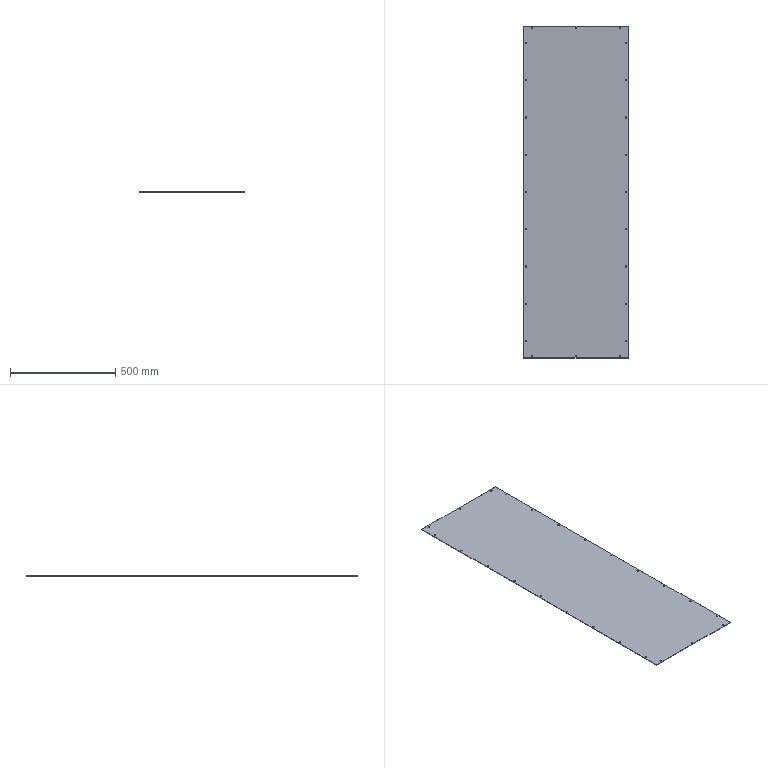Part | SolidWorks | 1 solid | 54 faces | box 494.5 x 1578 x 2 mm | volume 1559049 mm3 | cylinder 48 | plane 6 | commonest cylinder face diameters 6.5 x48